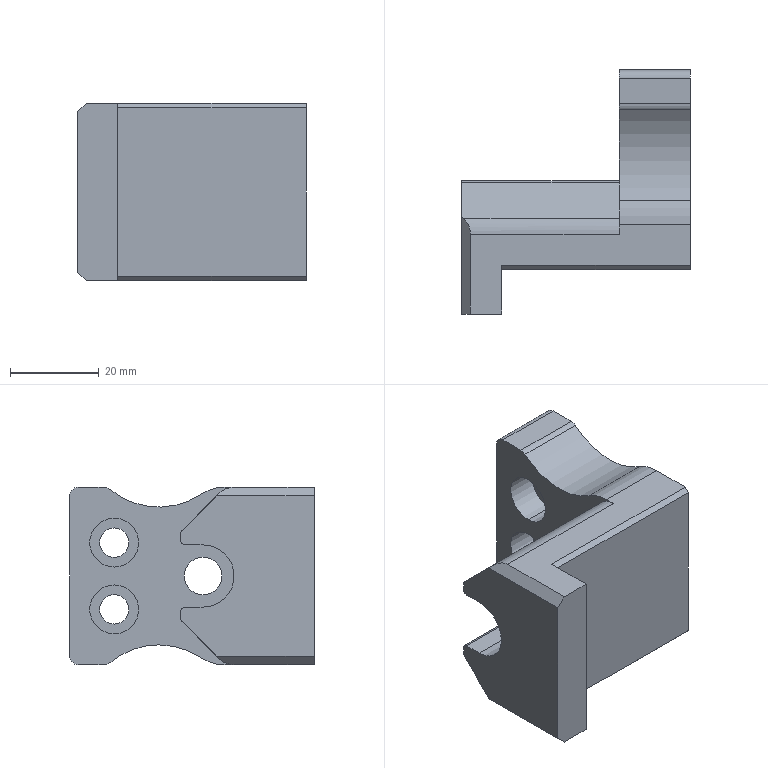Part | SolidWorks | features BaseBody 1 | 1 solid | 55 faces | box 51.5 x 55 x 40 mm | volume 46116 mm3 | cylinder 30 | plane 25 | commonest cylinder face diameters 2 x4 4 x4 6 x4 6.6 x4 11 x4 34 x3